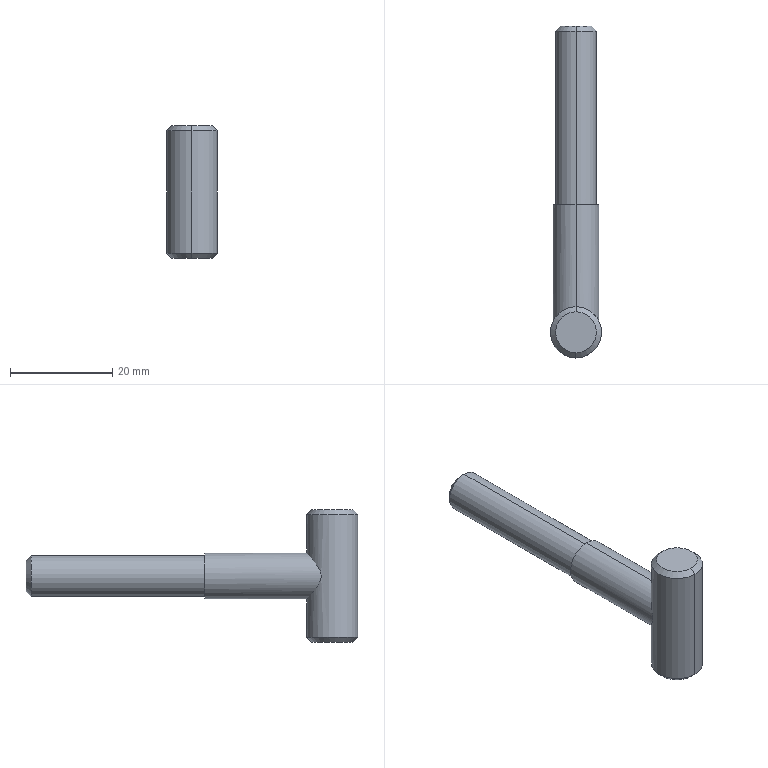Part | STEP file | Input 47 | 1 solid | 16 faces | box 10 x 65 x 26 mm | volume 5070 mm3 | cone 6 | cylinder 6 | plane 4 | commonest cylinder face diameters 8 x2 9 x2 10 x2